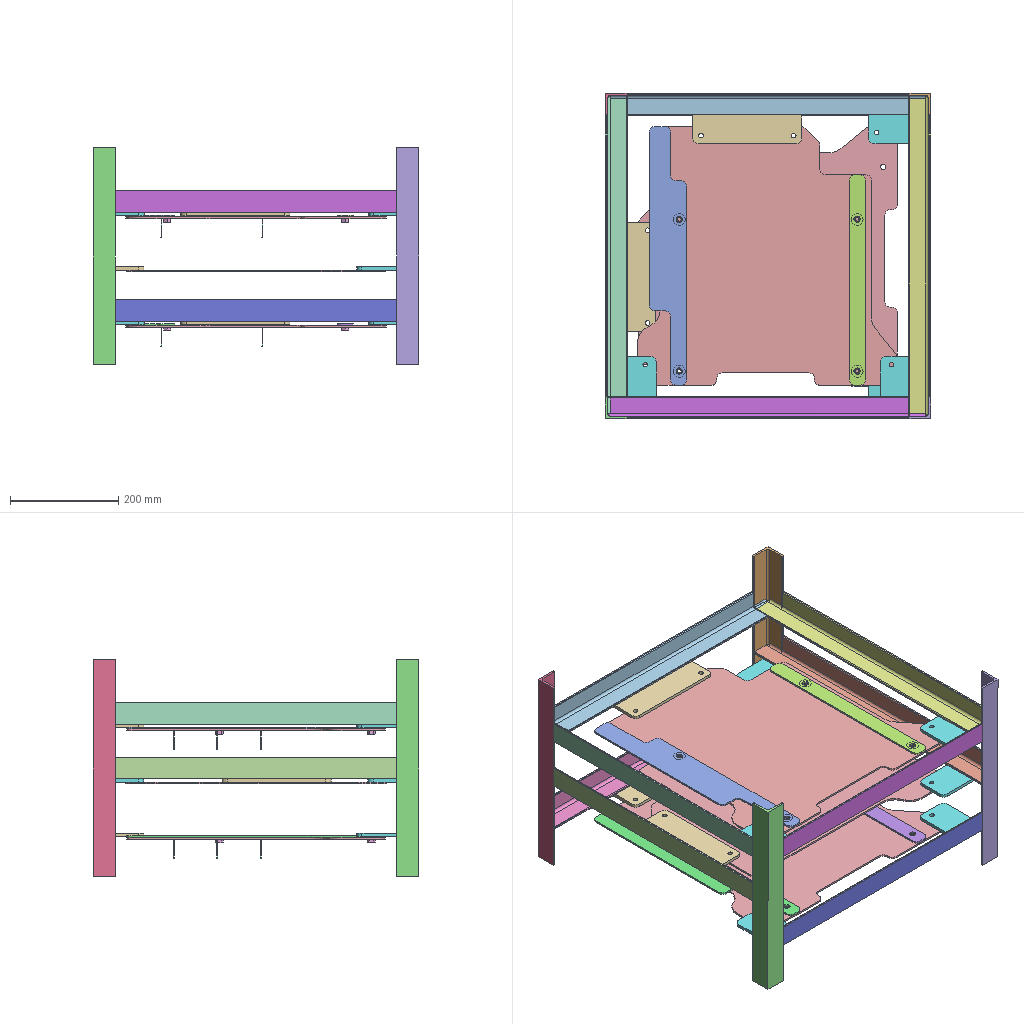Assembly | SolidWorks | 8 different items | 31 placed | box 600 x 600 x 400 mm
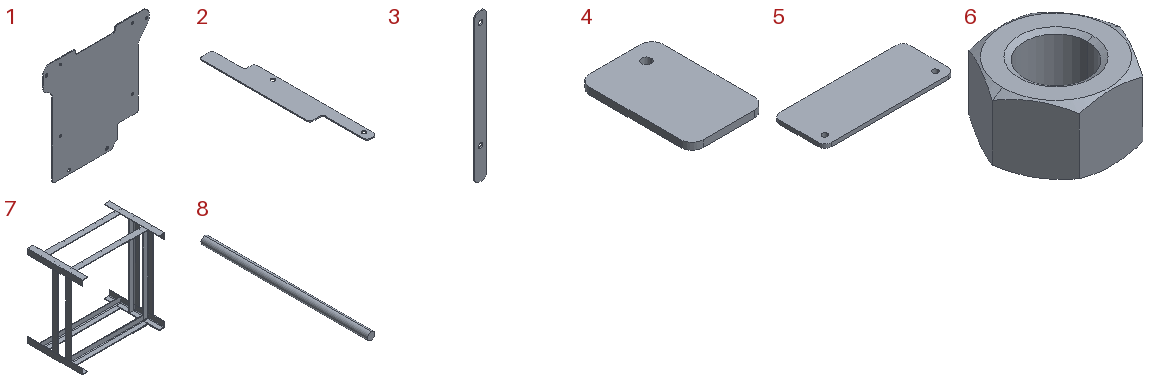Parts list (item | quantity | size | volume | features):
1 | x3 | 481 x 3.2 x 477 mm | 577173 mm3 | features FlatPattern 1, SMBaseFlange 1, SheetMetal 1
2 | x2 | 70 x 477 x 3.2 mm | 78713 mm3 | features FlatPattern 1, SMBaseFlange 1, SheetMetal 1
3 | x2 | 30 x 3.2 x 388 mm | 36249 mm3 | features FlatPattern 1, SMBaseFlange 1, SheetMetal 1
4 | x6 | 65 x 100 x 6 mm | 38144 mm3 | features FlatPattern 1, SMBaseFlange 1, SheetMetal 1
5 | x3 | 201 x 80 x 6 mm | 95284 mm3 | features FlatPattern 1, SMBaseFlange 1, SheetMetal 1
6 | x8 | 27.713 x 24 x 14.8 mm | 5071 mm3 | features RevCut 2, Chamfer 1, Extrusion 1, LPattern 1
7 | x1 | 600 x 400 x 600 mm | 1841733 mm3 | features 3DProfileFeature 1, WeldMemberFeat 1, WeldmentFeature 1
8 | x6 | 1.6 x 35 x 1.6 mm | 70.372 mm3 | features Extrusion 1
Mates (type | each side: item.copy, entity, surface, feature):
Coincident | 1.1 face plane | 2.1 face plane Base-Flange1
Concentric | 1.1 face cylinder | 2.1 face cylinder Base-Flange1 | 2 times
Coincident | 1.1 face plane | 3.1 face plane Base-Flange1
Concentric | 1.1 face cylinder | 3.1 face cylinder Base-Flange1 | 2 times
Concentric | 1.1 face cylinder | 6.1 face cone EndChamfer
Coincident | 1.1 face plane | 6.1 face plane BaseNut
Concentric | 1.1 face cylinder | 6.2 face cone EndChamfer
Coincident | 1.1 face plane | 6.2 face plane BaseNut
Concentric | 1.1 face cylinder | 6.3 face cone EndChamfer
Coincident | 1.1 face plane | 6.3 face plane BaseNut
Concentric | 1.1 face cylinder | 6.4 face cone EndChamfer
Coincident | 1.1 face plane | 6.4 face plane BaseNut
Parallel | 1.1 face plane | 6.1 face plane BaseNut
Parallel | 1.1 face plane | 6.2 face plane BaseNut
Parallel | 1.1 face plane | 6.3 face plane BaseNut
Parallel | 1.1 face plane | 6.4 face plane BaseNut
Coincident | 1.1 face plane | 8.1 face plane Boss-Extrude1
DistanceDim | 8.1 face cylinder Boss-Extrude1 | 1.1 face plane | 2 times
Coincident | 1.1 face plane | 8.2 face plane Boss-Extrude1
DistanceDim | 8.2 face cylinder Boss-Extrude1 | 1.1 face plane | 2 times
Coincident | 1.1 face plane | 8.3 face plane Boss-Extrude1
DistanceDim | 8.3 face cylinder Boss-Extrude1 | 1.1 face plane
DistanceDim | 8.2 face cylinder Boss-Extrude1 | 8.3 face cylinder Boss-Extrude1
DistanceDim | 7.1 face plane GB/T 9787-1988 hot-rolled equal angle 40 X 4(1) | 1.1 face plane
InPlace | 7.1 face plane GB/T 9787-1988 hot-rolled equal angle 40 X 4(1) | 4.1 plane
Coincident | 7.1 face plane GB/T 9787-1988 hot-rolled equal angle 40 X 4(1) | 4.2 face plane Base-Flange1
Concentric | 1.1 face cylinder | 4.2 face cylinder Base-Flange1
Coincident | 4.1 face plane Base-Flange1 | 4.2 face plane Base-Flange1
Parallel | 1.1 face plane | 7.1 face plane GB/T 9787-1988 hot-rolled equal angle 40 X 4(1) | 2 times
DistanceDim | 1.1 face plane | 7.1 face plane GB/T 9787-1988 hot-rolled equal angle 40 X 4(1)
InPlace | 7.1 face plane GB/T 9787-1988 hot-rolled equal angle 40 X 4(1) | 5.1 plane
Coincident | 7.1 face plane GB/T 9787-1988 hot-rolled equal angle 40 X 4(1) | 4.3 face plane Base-Flange1
DistanceDim | 4.3 face plane Base-Flange1 | 7.1 face plane GB/T 9787-1988 hot-rolled equal angle 40 X 4(1)
DistanceDim | 7.1 face plane GB/T 9787-1988 hot-rolled equal angle 40 X 4(1) | 4.3 face plane Base-Flange1
Coincident | 7.1 face plane GB/T 9787-1988 hot-rolled equal angle 40 X 4(1) | 4.4 face plane Base-Flange1
DistanceDim | 4.4 face plane Base-Flange1 | 7.1 face plane GB/T 9787-1988 hot-rolled equal angle 40 X 4(1) | 2 times
Coincident | 7.1 face plane GB/T 9787-1988 hot-rolled equal angle 40 X 4(1) | 5.2 face plane Base-Flange1
DistanceDim | 7.1 face plane GB/T 9787-1988 hot-rolled equal angle 40 X 4(1) | 5.2 face plane Base-Flange1 | 2 times
Coincident | 5.2 face plane Base-Flange1 | 1.2 face plane Base-Flange1
Concentric | 4.4 face cylinder Base-Flange1 | 1.2 face cylinder Base-Flange1